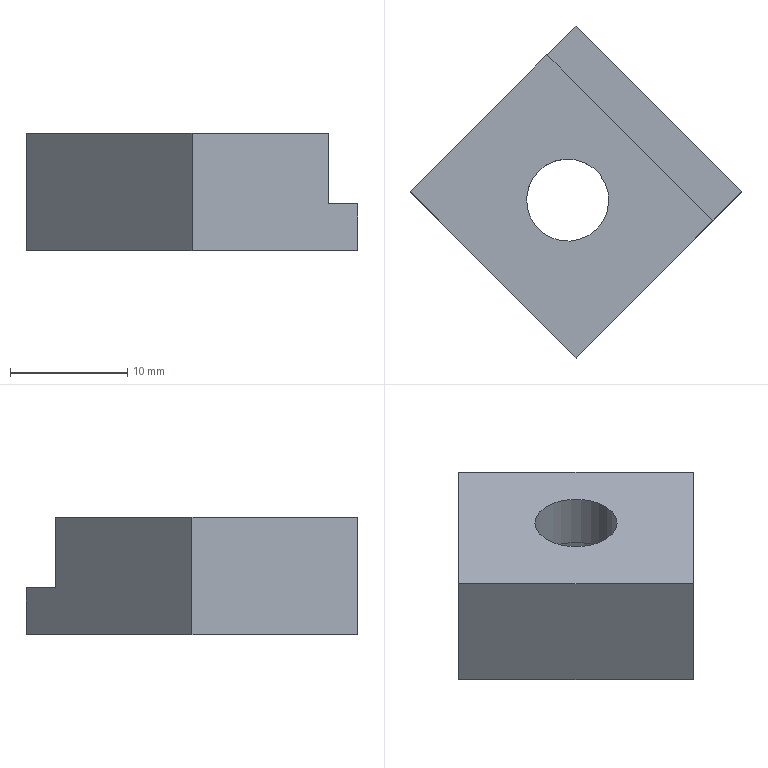Part | 1 solid | 13 faces | box 28.284 x 28.284 x 10 mm | volume 2884 mm3 | plane 9 | cylinder 4 | commonest cylinder face diameters 7 x2 11 x2
STEP:
#1=CARTESIAN_POINT('',(0.,0.,0.));
#2=DIRECTION('',(0.,0.,1.));
#3=DIRECTION('',(1.,0.,0.));
#4=AXIS2_PLACEMENT_3D('',#1,#2,#3);
#5=CARTESIAN_POINT('',(-358.688,26.59,-133.051));
#6=VERTEX_POINT('',#5);
#7=CARTESIAN_POINT('',(-350.91,18.812,-133.051));
#8=VERTEX_POINT('',#7);
#9=CARTESIAN_POINT('',(-354.799,22.701,-133.051));
#10=DIRECTION('',(0.,0.,1.));
#11=DIRECTION('',(-0.7071,0.7071,0.));
#12=AXIS2_PLACEMENT_3D('',#9,#10,#11);
#13=CIRCLE('',#12,5.5);
#14=CARTESIAN_POINT('',(-368.234,23.408,-133.051));
#15=DIRECTION('',(0.,0.,1.));
#16=DIRECTION('',(-0.7071,0.7071,0.));
#17=AXIS2_PLACEMENT_3D('',#14,#15,#16);
#18=PLANE('',#17);
#19=CARTESIAN_POINT('',(-10.,-9.));
#20=DIRECTION('',(1.,0.));
#21=AXIS2_PLACEMENT_2D('',#19,#20);
#22=CIRCLE('',#21,5.5);
#23=(GEOMETRIC_REPRESENTATION_CONTEXT(2)PARAMETRIC_REPRESENTATION_CONTEXT()REPRESENTATION_CONTEXT('',''));
#24=DEFINITIONAL_REPRESENTATION('',(#22),#23);
#25=PCURVE('',#18,#24);
#26=CARTESIAN_POINT('',(-354.799,22.701,-139.051));
#27=DIRECTION('',(0.,0.,1.));
#28=DIRECTION('',(0.7071,0.7071,0.));
#29=AXIS2_PLACEMENT_3D('',#26,#27,#28);
#30=CYLINDRICAL_SURFACE('',#29,5.5);
#31=CARTESIAN_POINT('',(1.571,6.));
#32=DIRECTION('',(1.,0.));
#33=VECTOR('',#32,1.);
#34=LINE('',#31,#33);
#35=(GEOMETRIC_REPRESENTATION_CONTEXT(2)PARAMETRIC_REPRESENTATION_CONTEXT()REPRESENTATION_CONTEXT('',''));
#36=DEFINITIONAL_REPRESENTATION('',(#34),#35);
#37=PCURVE('',#30,#36);
#38=SURFACE_CURVE('',#13,(#25,#37),.PCURVE_S1.);
#39=EDGE_CURVE('',#6,#8,#38,.T.);
#40=ORIENTED_EDGE('',*,*,#39,.T.);
#41=CARTESIAN_POINT('',(-354.799,22.701,-133.051));
#42=DIRECTION('',(0.,0.,1.));
#43=DIRECTION('',(-0.7071,0.7071,0.));
#44=AXIS2_PLACEMENT_3D('',#41,#42,#43);
#45=CIRCLE('',#44,5.5);
#46=CARTESIAN_POINT('',(-10.,-9.));
#47=DIRECTION('',(1.,0.));
#48=AXIS2_PLACEMENT_2D('',#46,#47);
#49=CIRCLE('',#48,5.5);
#50=(GEOMETRIC_REPRESENTATION_CONTEXT(2)PARAMETRIC_REPRESENTATION_CONTEXT()REPRESENTATION_CONTEXT('',''));
#51=DEFINITIONAL_REPRESENTATION('',(#49),#50);
#52=PCURVE('',#18,#51);
#53=CARTESIAN_POINT('',(-354.799,22.701,-139.051));
#54=DIRECTION('',(0.,0.,1.));
#55=DIRECTION('',(-0.7071,-0.7071,0.));
#56=AXIS2_PLACEMENT_3D('',#53,#54,#55);
#57=CYLINDRICAL_SURFACE('',#56,5.5);
#58=CARTESIAN_POINT('',(-1.571,6.));
#59=DIRECTION('',(1.,0.));
#60=VECTOR('',#59,1.);
#61=LINE('',#58,#60);
#62=(GEOMETRIC_REPRESENTATION_CONTEXT(2)PARAMETRIC_REPRESENTATION_CONTEXT()REPRESENTATION_CONTEXT('',''));
#63=DEFINITIONAL_REPRESENTATION('',(#61),#62);
#64=PCURVE('',#57,#63);
#65=SURFACE_CURVE('',#45,(#52,#64),.PCURVE_S1.);
#66=EDGE_CURVE('',#8,#6,#65,.T.);
#67=ORIENTED_EDGE('',*,*,#66,.T.);
#68=EDGE_LOOP('',(#40,#67));
#69=FACE_BOUND('',#68,.T.);
#70=CARTESIAN_POINT('',(-339.95,23.408,-133.051));
#71=VERTEX_POINT('',#70);
#72=CARTESIAN_POINT('',(-354.092,9.266,-133.051));
#73=VERTEX_POINT('',#72);
#74=CARTESIAN_POINT('',(-354.092,9.266,-133.051));
#75=DIRECTION('',(-0.7071,-0.7071,0.));
#76=VECTOR('',#75,1.);
#77=LINE('',#74,#76);
#78=CARTESIAN_POINT('',(-20.,0.));
#79=DIRECTION('',(0.,1.));
#80=VECTOR('',#79,1.);
#81=LINE('',#78,#80);
#82=(GEOMETRIC_REPRESENTATION_CONTEXT(2)PARAMETRIC_REPRESENTATION_CONTEXT()REPRESENTATION_CONTEXT('',''));
#83=DEFINITIONAL_REPRESENTATION('',(#81),#82);
#84=PCURVE('',#18,#83);
#85=CARTESIAN_POINT('',(1570.788,1934.145,521.628));
#86=DIRECTION('',(-0.7071,0.7071,0.));
#87=DIRECTION('',(0.7071,0.7071,0.));
#88=AXIS2_PLACEMENT_3D('',#85,#86,#87);
#89=PLANE('',#88);
#90=CARTESIAN_POINT('',(-2722.191,654.68));
#91=DIRECTION('',(-1.,0.));
#92=VECTOR('',#91,1.);
#93=LINE('',#90,#92);
#94=(GEOMETRIC_REPRESENTATION_CONTEXT(2)PARAMETRIC_REPRESENTATION_CONTEXT()REPRESENTATION_CONTEXT('',''));
#95=DEFINITIONAL_REPRESENTATION('',(#93),#94);
#96=PCURVE('',#89,#95);
#97=SURFACE_CURVE('',#77,(#84,#96),.PCURVE_S1.);
#98=EDGE_CURVE('',#71,#73,#97,.T.);
#99=ORIENTED_EDGE('',*,*,#98,.T.);
#100=CARTESIAN_POINT('',(-368.234,23.408,-133.051));
#101=VERTEX_POINT('',#100);
#102=CARTESIAN_POINT('',(-368.234,23.408,-133.051));
#103=DIRECTION('',(-0.7071,0.7071,0.));
#104=VECTOR('',#103,1.);
#105=LINE('',#102,#104);
#106=CARTESIAN_POINT('',(0.,0.));
#107=DIRECTION('',(1.,0.));
#108=VECTOR('',#107,1.);
#109=LINE('',#106,#108);
#110=(GEOMETRIC_REPRESENTATION_CONTEXT(2)PARAMETRIC_REPRESENTATION_CONTEXT()REPRESENTATION_CONTEXT('',''));
#111=DEFINITIONAL_REPRESENTATION('',(#109),#110);
#112=PCURVE('',#18,#111);
#113=CARTESIAN_POINT('',(-368.234,23.408,-123.051));
#114=DIRECTION('',(0.7071,0.7071,0.));
#115=DIRECTION('',(0.7071,-0.7071,0.));
#116=AXIS2_PLACEMENT_3D('',#113,#114,#115);
#117=PLANE('',#116);
#118=CARTESIAN_POINT('',(0.,10.));
#119=DIRECTION('',(-1.,0.));
#120=VECTOR('',#119,1.);
#121=LINE('',#118,#120);
#122=(GEOMETRIC_REPRESENTATION_CONTEXT(2)PARAMETRIC_REPRESENTATION_CONTEXT()REPRESENTATION_CONTEXT('',''));
#123=DEFINITIONAL_REPRESENTATION('',(#121),#122);
#124=PCURVE('',#117,#123);
#125=SURFACE_CURVE('',#105,(#112,#124),.PCURVE_S1.);
#126=EDGE_CURVE('',#73,#101,#125,.T.);
#127=ORIENTED_EDGE('',*,*,#126,.T.);
#128=CARTESIAN_POINT('',(-354.092,37.55,-133.051));
#129=VERTEX_POINT('',#128);
#130=CARTESIAN_POINT('',(-368.234,23.408,-133.051));
#131=DIRECTION('',(-0.7071,-0.7071,0.));
#132=VECTOR('',#131,1.);
#133=LINE('',#130,#132);
#134=CARTESIAN_POINT('',(0.,0.));
#135=DIRECTION('',(0.,1.));
#136=VECTOR('',#135,1.);
#137=LINE('',#134,#136);
#138=(GEOMETRIC_REPRESENTATION_CONTEXT(2)PARAMETRIC_REPRESENTATION_CONTEXT()REPRESENTATION_CONTEXT('',''));
#139=DEFINITIONAL_REPRESENTATION('',(#137),#138);
#140=PCURVE('',#18,#139);
#141=CARTESIAN_POINT('',(1556.646,1948.287,521.628));
#142=DIRECTION('',(-0.7071,0.7071,0.));
#143=DIRECTION('',(0.7071,0.7071,0.));
#144=AXIS2_PLACEMENT_3D('',#141,#142,#143);
#145=PLANE('',#144);
#146=CARTESIAN_POINT('',(-2722.191,654.68));
#147=DIRECTION('',(-1.,0.));
#148=VECTOR('',#147,1.);
#149=LINE('',#146,#148);
#150=(GEOMETRIC_REPRESENTATION_CONTEXT(2)PARAMETRIC_REPRESENTATION_CONTEXT()REPRESENTATION_CONTEXT('',''));
#151=DEFINITIONAL_REPRESENTATION('',(#149),#150);
#152=PCURVE('',#145,#151);
#153=SURFACE_CURVE('',#133,(#140,#152),.PCURVE_S1.);
#154=EDGE_CURVE('',#129,#101,#153,.T.);
#155=ORIENTED_EDGE('',*,*,#154,.F.);
#156=CARTESIAN_POINT('',(-354.092,37.55,-133.051));
#157=DIRECTION('',(-0.7071,0.7071,0.));
#158=VECTOR('',#157,1.);
#159=LINE('',#156,#158);
#160=CARTESIAN_POINT('',(0.,-20.));
#161=DIRECTION('',(1.,0.));
#162=VECTOR('',#161,1.);
#163=LINE('',#160,#162);
#164=(GEOMETRIC_REPRESENTATION_CONTEXT(2)PARAMETRIC_REPRESENTATION_CONTEXT()REPRESENTATION_CONTEXT('',''));
#165=DEFINITIONAL_REPRESENTATION('',(#163),#164);
#166=PCURVE('',#18,#165);
#167=CARTESIAN_POINT('',(-354.092,37.55,-133.051));
#168=DIRECTION('',(-0.7071,-0.7071,0.));
#169=DIRECTION('',(-0.7071,0.7071,0.));
#170=AXIS2_PLACEMENT_3D('',#167,#168,#169);
#171=PLANE('',#170);
#172=CARTESIAN_POINT('',(0.,0.));
#173=DIRECTION('',(1.,0.));
#174=VECTOR('',#173,1.);
#175=LINE('',#172,#174);
#176=(GEOMETRIC_REPRESENTATION_CONTEXT(2)PARAMETRIC_REPRESENTATION_CONTEXT()REPRESENTATION_CONTEXT('',''));
#177=DEFINITIONAL_REPRESENTATION('',(#175),#176);
#178=PCURVE('',#171,#177);
#179=SURFACE_CURVE('',#159,(#166,#178),.PCURVE_S1.);
#180=EDGE_CURVE('',#71,#129,#179,.T.);
#181=ORIENTED_EDGE('',*,*,#180,.F.);
#182=EDGE_LOOP('',(#99,#127,#155,#181));
#183=FACE_BOUND('',#182,.T.);
#184=ADVANCED_FACE('',(#69,#183),#18,.F.);
#185=CARTESIAN_POINT('',(-339.95,23.408,-129.051));
#186=VERTEX_POINT('',#185);
#187=CARTESIAN_POINT('',(-339.95,23.408,-133.051));
#188=DIRECTION('',(0.,0.,-1.));
#189=VECTOR('',#188,1.);
#190=LINE('',#187,#189);
#191=CARTESIAN_POINT('',(-20.,0.));
#192=DIRECTION('',(0.,1.));
#193=VECTOR('',#192,1.);
#194=LINE('',#191,#193);
#195=(GEOMETRIC_REPRESENTATION_CONTEXT(2)PARAMETRIC_REPRESENTATION_CONTEXT()REPRESENTATION_CONTEXT('',''));
#196=DEFINITIONAL_REPRESENTATION('',(#194),#195);
#197=PCURVE('',#171,#196);
#198=CARTESIAN_POINT('',(-2702.191,654.68));
#199=DIRECTION('',(0.,1.));
#200=VECTOR('',#199,1.);
#201=LINE('',#198,#200);
#202=(GEOMETRIC_REPRESENTATION_CONTEXT(2)PARAMETRIC_REPRESENTATION_CONTEXT()REPRESENTATION_CONTEXT('',''));
#203=DEFINITIONAL_REPRESENTATION('',(#201),#202);
#204=PCURVE('',#89,#203);
#205=SURFACE_CURVE('',#190,(#197,#204),.PCURVE_S1.);
#206=EDGE_CURVE('',#186,#71,#205,.T.);
#207=ORIENTED_EDGE('',*,*,#206,.T.);
#208=ORIENTED_EDGE('',*,*,#180,.T.);
#209=CARTESIAN_POINT('',(-354.092,37.55,-129.051));
#210=VERTEX_POINT('',#209);
#211=CARTESIAN_POINT('',(-354.092,37.55,-133.051));
#212=DIRECTION('',(0.,0.,-1.));
#213=VECTOR('',#212,1.);
#214=LINE('',#211,#213);
#215=CARTESIAN_POINT('',(0.,0.));
#216=DIRECTION('',(0.,1.));
#217=VECTOR('',#216,1.);
#218=LINE('',#215,#217);
#219=(GEOMETRIC_REPRESENTATION_CONTEXT(2)PARAMETRIC_REPRESENTATION_CONTEXT()REPRESENTATION_CONTEXT('',''));
#220=DEFINITIONAL_REPRESENTATION('',(#218),#219);
#221=PCURVE('',#171,#220);
#222=CARTESIAN_POINT('',(-2702.191,654.68));
#223=DIRECTION('',(0.,1.));
#224=VECTOR('',#223,1.);
#225=LINE('',#222,#224);
#226=(GEOMETRIC_REPRESENTATION_CONTEXT(2)PARAMETRIC_REPRESENTATION_CONTEXT()REPRESENTATION_CONTEXT('',''));
#227=DEFINITIONAL_REPRESENTATION('',(#225),#226);
#228=PCURVE('',#145,#227);
#229=SURFACE_CURVE('',#214,(#221,#228),.PCURVE_S1.);
#230=EDGE_CURVE('',#210,#129,#229,.T.);
#231=ORIENTED_EDGE('',*,*,#230,.F.);
#232=CARTESIAN_POINT('',(-354.092,37.55,-129.051));
#233=DIRECTION('',(-0.7071,0.7071,0.));
#234=VECTOR('',#233,1.);
#235=LINE('',#232,#234);
#236=CARTESIAN_POINT('',(0.,-4.));
#237=DIRECTION('',(1.,0.));
#238=VECTOR('',#237,1.);
#239=LINE('',#236,#238);
#240=(GEOMETRIC_REPRESENTATION_CONTEXT(2)PARAMETRIC_REPRESENTATION_CONTEXT()REPRESENTATION_CONTEXT('',''));
#241=DEFINITIONAL_REPRESENTATION('',(#239),#240);
#242=PCURVE('',#171,#241);
#243=CARTESIAN_POINT('',(-354.092,37.55,-129.051));
#244=DIRECTION('',(0.,0.,-1.));
#245=DIRECTION('',(0.7071,-0.7071,0.));
#246=AXIS2_PLACEMENT_3D('',#243,#244,#245);
#247=PLANE('',#246);
#248=CARTESIAN_POINT('',(0.,0.));
#249=DIRECTION('',(-1.,0.));
#250=VECTOR('',#249,1.);
#251=LINE('',#248,#250);
#252=(GEOMETRIC_REPRESENTATION_CONTEXT(2)PARAMETRIC_REPRESENTATION_CONTEXT()REPRESENTATION_CONTEXT('',''));
#253=DEFINITIONAL_REPRESENTATION('',(#251),#252);
#254=PCURVE('',#247,#253);
#255=SURFACE_CURVE('',#235,(#242,#254),.PCURVE_S1.);
#256=EDGE_CURVE('',#186,#210,#255,.T.);
#257=ORIENTED_EDGE('',*,*,#256,.F.);
#258=EDGE_LOOP('',(#207,#208,#231,#257));
#259=FACE_BOUND('',#258,.T.);
#260=ADVANCED_FACE('',(#259),#171,.F.);
#261=CARTESIAN_POINT('',(-342.424,20.933,-129.051));
#262=VERTEX_POINT('',#261);
#263=CARTESIAN_POINT('',(-339.95,23.408,-129.051));
#264=DIRECTION('',(0.7071,0.7071,0.));
#265=VECTOR('',#264,1.);
#266=LINE('',#263,#265);
#267=CARTESIAN_POINT('',(20.,0.));
#268=DIRECTION('',(0.,-1.));
#269=VECTOR('',#268,1.);
#270=LINE('',#267,#269);
#271=(GEOMETRIC_REPRESENTATION_CONTEXT(2)PARAMETRIC_REPRESENTATION_CONTEXT()REPRESENTATION_CONTEXT('',''));
#272=DEFINITIONAL_REPRESENTATION('',(#270),#271);
#273=PCURVE('',#247,#272);
#274=CARTESIAN_POINT('',(-2702.191,650.68));
#275=DIRECTION('',(1.,0.));
#276=VECTOR('',#275,1.);
#277=LINE('',#274,#276);
#278=(GEOMETRIC_REPRESENTATION_CONTEXT(2)PARAMETRIC_REPRESENTATION_CONTEXT()REPRESENTATION_CONTEXT('',''));
#279=DEFINITIONAL_REPRESENTATION('',(#277),#278);
#280=PCURVE('',#89,#279);
#281=SURFACE_CURVE('',#266,(#273,#280),.PCURVE_S1.);
#282=EDGE_CURVE('',#262,#186,#281,.T.);
#283=ORIENTED_EDGE('',*,*,#282,.T.);
#284=ORIENTED_EDGE('',*,*,#256,.T.);
#285=CARTESIAN_POINT('',(-356.567,35.075,-129.051));
#286=VERTEX_POINT('',#285);
#287=CARTESIAN_POINT('',(-354.092,37.55,-129.051));
#288=DIRECTION('',(0.7071,0.7071,0.));
#289=VECTOR('',#288,1.);
#290=LINE('',#287,#289);
#291=CARTESIAN_POINT('',(0.,0.));
#292=DIRECTION('',(0.,-1.));
#293=VECTOR('',#292,1.);
#294=LINE('',#291,#293);
#295=(GEOMETRIC_REPRESENTATION_CONTEXT(2)PARAMETRIC_REPRESENTATION_CONTEXT()REPRESENTATION_CONTEXT('',''));
#296=DEFINITIONAL_REPRESENTATION('',(#294),#295);
#297=PCURVE('',#247,#296);
#298=CARTESIAN_POINT('',(-2702.191,650.68));
#299=DIRECTION('',(1.,0.));
#300=VECTOR('',#299,1.);
#301=LINE('',#298,#300);
#302=(GEOMETRIC_REPRESENTATION_CONTEXT(2)PARAMETRIC_REPRESENTATION_CONTEXT()REPRESENTATION_CONTEXT('',''));
#303=DEFINITIONAL_REPRESENTATION('',(#301),#302);
#304=PCURVE('',#145,#303);
#305=SURFACE_CURVE('',#290,(#297,#304),.PCURVE_S1.);
#306=EDGE_CURVE('',#286,#210,#305,.T.);
#307=ORIENTED_EDGE('',*,*,#306,.F.);
#308=CARTESIAN_POINT('',(-356.567,35.075,-129.051));
#309=DIRECTION('',(-0.7071,0.7071,0.));
#310=VECTOR('',#309,1.);
#311=LINE('',#308,#310);
#312=CARTESIAN_POINT('',(0.,3.5));
#313=DIRECTION('',(-1.,0.));
#314=VECTOR('',#313,1.);
#315=LINE('',#312,#314);
#316=(GEOMETRIC_REPRESENTATION_CONTEXT(2)PARAMETRIC_REPRESENTATION_CONTEXT()REPRESENTATION_CONTEXT('',''));
#317=DEFINITIONAL_REPRESENTATION('',(#315),#316);
#318=PCURVE('',#247,#317);
#319=CARTESIAN_POINT('',(-356.567,35.075,-129.051));
#320=DIRECTION('',(-0.7071,-0.7071,0.));
#321=DIRECTION('',(-0.7071,0.7071,0.));
#322=AXIS2_PLACEMENT_3D('',#319,#320,#321);
#323=PLANE('',#322);
#324=CARTESIAN_POINT('',(0.,0.));
#325=DIRECTION('',(1.,0.));
#326=VECTOR('',#325,1.);
#327=LINE('',#324,#326);
#328=(GEOMETRIC_REPRESENTATION_CONTEXT(2)PARAMETRIC_REPRESENTATION_CONTEXT()REPRESENTATION_CONTEXT('',''));
#329=DEFINITIONAL_REPRESENTATION('',(#327),#328);
#330=PCURVE('',#323,#329);
#331=SURFACE_CURVE('',#311,(#318,#330),.PCURVE_S1.);
#332=EDGE_CURVE('',#262,#286,#331,.T.);
#333=ORIENTED_EDGE('',*,*,#332,.F.);
#334=EDGE_LOOP('',(#283,#284,#307,#333));
#335=FACE_BOUND('',#334,.T.);
#336=ADVANCED_FACE('',(#335),#247,.F.);
#337=CARTESIAN_POINT('',(-342.424,20.933,-123.051));
#338=VERTEX_POINT('',#337);
#339=CARTESIAN_POINT('',(-342.424,20.933,-129.051));
#340=DIRECTION('',(0.,0.,-1.));
#341=VECTOR('',#340,1.);
#342=LINE('',#339,#341);
#343=CARTESIAN_POINT('',(-20.,0.));
#344=DIRECTION('',(0.,1.));
#345=VECTOR('',#344,1.);
#346=LINE('',#343,#345);
#347=(GEOMETRIC_REPRESENTATION_CONTEXT(2)PARAMETRIC_REPRESENTATION_CONTEXT()REPRESENTATION_CONTEXT('',''));
#348=DEFINITIONAL_REPRESENTATION('',(#346),#347);
#349=PCURVE('',#323,#348);
#350=CARTESIAN_POINT('',(-2705.691,650.68));
#351=DIRECTION('',(0.,1.));
#352=VECTOR('',#351,1.);
#353=LINE('',#350,#352);
#354=(GEOMETRIC_REPRESENTATION_CONTEXT(2)PARAMETRIC_REPRESENTATION_CONTEXT()REPRESENTATION_CONTEXT('',''));
#355=DEFINITIONAL_REPRESENTATION('',(#353),#354);
#356=PCURVE('',#89,#355);
#357=SURFACE_CURVE('',#342,(#349,#356),.PCURVE_S1.);
#358=EDGE_CURVE('',#338,#262,#357,.T.);
#359=ORIENTED_EDGE('',*,*,#358,.T.);
#360=ORIENTED_EDGE('',*,*,#332,.T.);
#361=CARTESIAN_POINT('',(-356.567,35.075,-123.051));
#362=VERTEX_POINT('',#361);
#363=CARTESIAN_POINT('',(-356.567,35.075,-129.051));
#364=DIRECTION('',(0.,0.,-1.));
#365=VECTOR('',#364,1.);
#366=LINE('',#363,#365);
#367=CARTESIAN_POINT('',(0.,0.));
#368=DIRECTION('',(0.,1.));
#369=VECTOR('',#368,1.);
#370=LINE('',#367,#369);
#371=(GEOMETRIC_REPRESENTATION_CONTEXT(2)PARAMETRIC_REPRESENTATION_CONTEXT()REPRESENTATION_CONTEXT('',''));
#372=DEFINITIONAL_REPRESENTATION('',(#370),#371);
#373=PCURVE('',#323,#372);
#374=CARTESIAN_POINT('',(-2705.691,650.68));
#375=DIRECTION('',(0.,1.));
#376=VECTOR('',#375,1.);
#377=LINE('',#374,#376);
#378=(GEOMETRIC_REPRESENTATION_CONTEXT(2)PARAMETRIC_REPRESENTATION_CONTEXT()REPRESENTATION_CONTEXT('',''));
#379=DEFINITIONAL_REPRESENTATION('',(#377),#378);
#380=PCURVE('',#145,#379);
#381=SURFACE_CURVE('',#366,(#373,#380),.PCURVE_S1.);
#382=EDGE_CURVE('',#362,#286,#381,.T.);
#383=ORIENTED_EDGE('',*,*,#382,.F.);
#384=CARTESIAN_POINT('',(-356.567,35.075,-123.051));
#385=DIRECTION('',(-0.7071,0.7071,0.));
#386=VECTOR('',#385,1.);
#387=LINE('',#384,#386);
#388=CARTESIAN_POINT('',(0.,-6.));
#389=DIRECTION('',(1.,0.));
#390=VECTOR('',#389,1.);
#391=LINE('',#388,#390);
#392=(GEOMETRIC_REPRESENTATION_CONTEXT(2)PARAMETRIC_REPRESENTATION_CONTEXT()REPRESENTATION_CONTEXT('',''));
#393=DEFINITIONAL_REPRESENTATION('',(#391),#392);
#394=PCURVE('',#323,#393);
#395=CARTESIAN_POINT('',(-356.567,35.075,-123.051));
#396=DIRECTION('',(0.,0.,-1.));
#397=DIRECTION('',(0.7071,-0.7071,0.));
#398=AXIS2_PLACEMENT_3D('',#395,#396,#397);
#399=PLANE('',#398);
#400=CARTESIAN_POINT('',(0.,0.));
#401=DIRECTION('',(-1.,0.));
#402=VECTOR('',#401,1.);
#403=LINE('',#400,#402);
#404=(GEOMETRIC_REPRESENTATION_CONTEXT(2)PARAMETRIC_REPRESENTATION_CONTEXT()REPRESENTATION_CONTEXT('',''));
#405=DEFINITIONAL_REPRESENTATION('',(#403),#404);
#406=PCURVE('',#399,#405);
#407=SURFACE_CURVE('',#387,(#394,#406),.PCURVE_S1.);
#408=EDGE_CURVE('',#338,#362,#407,.T.);
#409=ORIENTED_EDGE('',*,*,#408,.F.);
#410=EDGE_LOOP('',(#359,#360,#383,#409));
#411=FACE_BOUND('',#410,.T.);
#412=ADVANCED_FACE('',(#411),#323,.F.);
#413=CARTESIAN_POINT('',(-357.274,25.176,-123.051));
#414=VERTEX_POINT('',#413);
#415=CARTESIAN_POINT('',(-352.324,20.226,-123.051));
#416=VERTEX_POINT('',#415);
#417=CARTESIAN_POINT('',(-354.799,22.701,-123.051));
#418=DIRECTION('',(0.,0.,-1.));
#419=DIRECTION('',(-0.7071,0.7071,0.));
#420=AXIS2_PLACEMENT_3D('',#417,#418,#419);
#421=CIRCLE('',#420,3.5);
#422=CARTESIAN_POINT('',(10.,7.5));
#423=DIRECTION('',(-1.,0.));
#424=AXIS2_PLACEMENT_2D('',#422,#423);
#425=CIRCLE('',#424,3.5);
#426=(GEOMETRIC_REPRESENTATION_CONTEXT(2)PARAMETRIC_REPRESENTATION_CONTEXT()REPRESENTATION_CONTEXT('',''));
#427=DEFINITIONAL_REPRESENTATION('',(#425),#426);
#428=PCURVE('',#399,#427);
#429=CARTESIAN_POINT('',(-354.799,22.701,-39.051));
#430=DIRECTION('',(0.,0.,1.));
#431=DIRECTION('',(-0.7071,-0.7071,0.));
#432=AXIS2_PLACEMENT_3D('',#429,#430,#431);
#433=CYLINDRICAL_SURFACE('',#432,3.5);
#434=CARTESIAN_POINT('',(4.712,-84.));
#435=DIRECTION('',(-1.,0.));
#436=VECTOR('',#435,1.);
#437=LINE('',#434,#436);
#438=(GEOMETRIC_REPRESENTATION_CONTEXT(2)PARAMETRIC_REPRESENTATION_CONTEXT()REPRESENTATION_CONTEXT('',''));
#439=DEFINITIONAL_REPRESENTATION('',(#437),#438);
#440=PCURVE('',#433,#439);
#441=SURFACE_CURVE('',#421,(#428,#440),.PCURVE_S1.);
#442=EDGE_CURVE('',#414,#416,#441,.T.);
#443=ORIENTED_EDGE('',*,*,#442,.T.);
#444=CARTESIAN_POINT('',(-354.799,22.701,-123.051));
#445=DIRECTION('',(0.,0.,-1.));
#446=DIRECTION('',(-0.7071,0.7071,0.));
#447=AXIS2_PLACEMENT_3D('',#444,#445,#446);
#448=CIRCLE('',#447,3.5);
#449=CARTESIAN_POINT('',(10.,7.5));
#450=DIRECTION('',(-1.,0.));
#451=AXIS2_PLACEMENT_2D('',#449,#450);
#452=CIRCLE('',#451,3.5);
#453=(GEOMETRIC_REPRESENTATION_CONTEXT(2)PARAMETRIC_REPRESENTATION_CONTEXT()REPRESENTATION_CONTEXT('',''));
#454=DEFINITIONAL_REPRESENTATION('',(#452),#453);
#455=PCURVE('',#399,#454);
#456=CARTESIAN_POINT('',(-354.799,22.701,-39.051));
#457=DIRECTION('',(0.,0.,1.));
#458=DIRECTION('',(0.7071,0.7071,0.));
#459=AXIS2_PLACEMENT_3D('',#456,#457,#458);
#460=CYLINDRICAL_SURFACE('',#459,3.5);
#461=CARTESIAN_POINT('',(7.854,-84.));
#462=DIRECTION('',(-1.,0.));
#463=VECTOR('',#462,1.);
#464=LINE('',#461,#463);
#465=(GEOMETRIC_REPRESENTATION_CONTEXT(2)PARAMETRIC_REPRESENTATION_CONTEXT()REPRESENTATION_CONTEXT('',''));
#466=DEFINITIONAL_REPRESENTATION('',(#464),#465);
#467=PCURVE('',#460,#466);
#468=SURFACE_CURVE('',#448,(#455,#467),.PCURVE_S1.);
#469=EDGE_CURVE('',#416,#414,#468,.T.);
#470=ORIENTED_EDGE('',*,*,#469,.T.);
#471=EDGE_LOOP('',(#443,#470));
#472=FACE_BOUND('',#471,.T.);
#473=CARTESIAN_POINT('',(-354.092,9.266,-123.051));
#474=VERTEX_POINT('',#473);
#475=CARTESIAN_POINT('',(-342.424,20.933,-123.051));
#476=DIRECTION('',(0.7071,0.7071,0.));
#477=VECTOR('',#476,1.);
#478=LINE('',#475,#477);
#479=CARTESIAN_POINT('',(20.,0.));
#480=DIRECTION('',(0.,-1.));
#481=VECTOR('',#480,1.);
#482=LINE('',#479,#481);
#483=(GEOMETRIC_REPRESENTATION_CONTEXT(2)PARAMETRIC_REPRESENTATION_CONTEXT()REPRESENTATION_CONTEXT('',''));
#484=DEFINITIONAL_REPRESENTATION('',(#482),#483);
#485=PCURVE('',#399,#484);
#486=CARTESIAN_POINT('',(-2705.691,644.68));
#487=DIRECTION('',(1.,0.));
#488=VECTOR('',#487,1.);
#489=LINE('',#486,#488);
#490=(GEOMETRIC_REPRESENTATION_CONTEXT(2)PARAMETRIC_REPRESENTATION_CONTEXT()REPRESENTATION_CONTEXT('',''));
#491=DEFINITIONAL_REPRESENTATION('',(#489),#490);
#492=PCURVE('',#89,#491);
#493=SURFACE_CURVE('',#478,(#485,#492),.PCURVE_S1.);
#494=EDGE_CURVE('',#474,#338,#493,.T.);
#495=ORIENTED_EDGE('',*,*,#494,.T.);
#496=ORIENTED_EDGE('',*,*,#408,.T.);
#497=CARTESIAN_POINT('',(-368.234,23.408,-123.051));
#498=VERTEX_POINT('',#497);
#499=CARTESIAN_POINT('',(-356.567,35.075,-123.051));
#500=DIRECTION('',(0.7071,0.7071,0.));
#501=VECTOR('',#500,1.);
#502=LINE('',#499,#501);
#503=CARTESIAN_POINT('',(0.,0.));
#504=DIRECTION('',(0.,-1.));
#505=VECTOR('',#504,1.);
#506=LINE('',#503,#505);
#507=(GEOMETRIC_REPRESENTATION_CONTEXT(2)PARAMETRIC_REPRESENTATION_CONTEXT()REPRESENTATION_CONTEXT('',''));
#508=DEFINITIONAL_REPRESENTATION('',(#506),#507);
#509=PCURVE('',#399,#508);
#510=CARTESIAN_POINT('',(-2705.691,644.68));
#511=DIRECTION('',(1.,0.));
#512=VECTOR('',#511,1.);
#513=LINE('',#510,#512);
#514=(GEOMETRIC_REPRESENTATION_CONTEXT(2)PARAMETRIC_REPRESENTATION_CONTEXT()REPRESENTATION_CONTEXT('',''));
#515=DEFINITIONAL_REPRESENTATION('',(#513),#514);
#516=PCURVE('',#145,#515);
#517=SURFACE_CURVE('',#502,(#509,#516),.PCURVE_S1.);
#518=EDGE_CURVE('',#498,#362,#517,.T.);
#519=ORIENTED_EDGE('',*,*,#518,.F.);
#520=CARTESIAN_POINT('',(-368.234,23.408,-123.051));
#521=DIRECTION('',(-0.7071,0.7071,0.));
#522=VECTOR('',#521,1.);
#523=LINE('',#520,#522);
#524=CARTESIAN_POINT('',(0.,16.5));
#525=DIRECTION('',(-1.,0.));
#526=VECTOR('',#525,1.);
#527=LINE('',#524,#526);
#528=(GEOMETRIC_REPRESENTATION_CONTEXT(2)PARAMETRIC_REPRESENTATION_CONTEXT()REPRESENTATION_CONTEXT('',''));
#529=DEFINITIONAL_REPRESENTATION('',(#527),#528);
#530=PCURVE('',#399,#529);
#531=CARTESIAN_POINT('',(0.,0.));
#532=DIRECTION('',(-1.,0.));
#533=VECTOR('',#532,1.);
#534=LINE('',#531,#533);
#535=(GEOMETRIC_REPRESENTATION_CONTEXT(2)PARAMETRIC_REPRESENTATION_CONTEXT()REPRESENTATION_CONTEXT('',''));
#536=DEFINITIONAL_REPRESENTATION('',(#534),#535);
#537=PCURVE('',#117,#536);
#538=SURFACE_CURVE('',#523,(#530,#537),.PCURVE_S1.);
#539=EDGE_CURVE('',#474,#498,#538,.T.);
#540=ORIENTED_EDGE('',*,*,#539,.F.);
#541=EDGE_LOOP('',(#495,#496,#519,#540));
#542=FACE_BOUND('',#541,.T.);
#543=ADVANCED_FACE('',(#472,#542),#399,.F.);
#544=CARTESIAN_POINT('',(-354.092,9.266,-123.051));
#545=DIRECTION('',(0.,0.,1.));
#546=VECTOR('',#545,1.);
#547=LINE('',#544,#546);
#548=CARTESIAN_POINT('',(20.,0.));
#549=DIRECTION('',(0.,-1.));
#550=VECTOR('',#549,1.);
#551=LINE('',#548,#550);
#552=(GEOMETRIC_REPRESENTATION_CONTEXT(2)PARAMETRIC_REPRESENTATION_CONTEXT()REPRESENTATION_CONTEXT('',''));
#553=DEFINITIONAL_REPRESENTATION('',(#551),#552);
#554=PCURVE('',#117,#553);
#555=CARTESIAN_POINT('',(-2722.191,644.68));
#556=DIRECTION('',(0.,-1.));
#557=VECTOR('',#556,1.);
#558=LINE('',#555,#557);
#559=(GEOMETRIC_REPRESENTATION_CONTEXT(2)PARAMETRIC_REPRESENTATION_CONTEXT()REPRESENTATION_CONTEXT('',''));
#560=DEFINITIONAL_REPRESENTATION('',(#558),#559);
#561=PCURVE('',#89,#560);
#562=SURFACE_CURVE('',#547,(#554,#561),.PCURVE_S1.);
#563=EDGE_CURVE('',#73,#474,#562,.T.);
#564=ORIENTED_EDGE('',*,*,#563,.T.);
#565=ORIENTED_EDGE('',*,*,#539,.T.);
#566=CARTESIAN_POINT('',(-368.234,23.408,-123.051));
#567=DIRECTION('',(0.,0.,1.));
#568=VECTOR('',#567,1.);
#569=LINE('',#566,#568);
#570=CARTESIAN_POINT('',(0.,0.));
#571=DIRECTION('',(0.,-1.));
#572=VECTOR('',#571,1.);
#573=LINE('',#570,#572);
#574=(GEOMETRIC_REPRESENTATION_CONTEXT(2)PARAMETRIC_REPRESENTATION_CONTEXT()REPRESENTATION_CONTEXT('',''));
#575=DEFINITIONAL_REPRESENTATION('',(#573),#574);
#576=PCURVE('',#117,#575);
#577=CARTESIAN_POINT('',(-2722.191,644.68));
#578=DIRECTION('',(0.,-1.));
#579=VECTOR('',#578,1.);
#580=LINE('',#577,#579);
#581=(GEOMETRIC_REPRESENTATION_CONTEXT(2)PARAMETRIC_REPRESENTATION_CONTEXT()REPRESENTATION_CONTEXT('',''));
#582=DEFINITIONAL_REPRESENTATION('',(#580),#581);
#583=PCURVE('',#145,#582);
#584=SURFACE_CURVE('',#569,(#576,#583),.PCURVE_S1.);
#585=EDGE_CURVE('',#101,#498,#584,.T.);
#586=ORIENTED_EDGE('',*,*,#585,.F.);
#587=ORIENTED_EDGE('',*,*,#126,.F.);
#588=EDGE_LOOP('',(#564,#565,#586,#587));
#589=FACE_BOUND('',#588,.T.);
#590=ADVANCED_FACE('',(#589),#117,.F.);
#591=ORIENTED_EDGE('',*,*,#154,.T.);
#592=ORIENTED_EDGE('',*,*,#585,.T.);
#593=ORIENTED_EDGE('',*,*,#518,.T.);
#594=ORIENTED_EDGE('',*,*,#382,.T.);
#595=ORIENTED_EDGE('',*,*,#306,.T.);
#596=ORIENTED_EDGE('',*,*,#230,.T.);
#597=EDGE_LOOP('',(#591,#592,#593,#594,#595,#596));
#598=FACE_BOUND('',#597,.T.);
#599=ADVANCED_FACE('',(#598),#145,.T.);
#600=ORIENTED_EDGE('',*,*,#98,.F.);
#601=ORIENTED_EDGE('',*,*,#206,.F.);
#602=ORIENTED_EDGE('',*,*,#282,.F.);
#603=ORIENTED_EDGE('',*,*,#358,.F.);
#604=ORIENTED_EDGE('',*,*,#494,.F.);
#605=ORIENTED_EDGE('',*,*,#563,.F.);
#606=EDGE_LOOP('',(#600,#601,#602,#603,#604,#605));
#607=FACE_BOUND('',#606,.T.);
#608=ADVANCED_FACE('',(#607),#89,.F.);
#609=CARTESIAN_POINT('',(-357.274,25.176,-127.551));
#610=VERTEX_POINT('',#609);
#611=CARTESIAN_POINT('',(-352.324,20.226,-127.551));
#612=VERTEX_POINT('',#611);
#613=CARTESIAN_POINT('',(-354.799,22.701,-127.551));
#614=DIRECTION('',(0.,0.,-1.));
#615=DIRECTION('',(-0.7071,0.7071,0.));
#616=AXIS2_PLACEMENT_3D('',#613,#614,#615);
#617=CIRCLE('',#616,3.5);
#618=CARTESIAN_POINT('',(4.712,-88.5));
#619=DIRECTION('',(-1.,0.));
#620=VECTOR('',#619,1.);
#621=LINE('',#618,#620);
#622=(GEOMETRIC_REPRESENTATION_CONTEXT(2)PARAMETRIC_REPRESENTATION_CONTEXT()REPRESENTATION_CONTEXT('',''));
#623=DEFINITIONAL_REPRESENTATION('',(#621),#622);
#624=PCURVE('',#433,#623);
#625=CARTESIAN_POINT('',(-354.799,22.701,-127.551));
#626=DIRECTION('',(0.,0.,1.));
#627=DIRECTION('',(-0.7071,0.7071,0.));
#628=AXIS2_PLACEMENT_3D('',#625,#626,#627);
#629=PLANE('',#628);
#630=CARTESIAN_POINT('',(3.5,0.));
#631=CARTESIAN_POINT('',(3.5,-6.062));
#632=CARTESIAN_POINT('',(-1.75,-3.031));
#633=CARTESIAN_POINT('',(-7.,0.));
#634=CARTESIAN_POINT('',(-1.75,3.031));
#635=CARTESIAN_POINT('',(3.5,6.062));
#636=CARTESIAN_POINT('',(3.5,0.));
#637=(BOUNDED_CURVE()B_SPLINE_CURVE(2,(#630,#631,#632,#633,#634,#635,#636),.UNSPECIFIED.,.T.,.F.)B_SPLINE_CURVE_WITH_KNOTS((1,2,2,2,2,1),(-2.094,0.,2.094,4.189,6.283,8.378),.UNSPECIFIED.)CURVE()GEOMETRIC_REPRESENTATION_ITEM()RATIONAL_B_SPLINE_CURVE((1.,0.5,1.,0.5,1.,0.5,1.))REPRESENTATION_ITEM(''));
#638=(GEOMETRIC_REPRESENTATION_CONTEXT(2)PARAMETRIC_REPRESENTATION_CONTEXT()REPRESENTATION_CONTEXT('',''));
#639=DEFINITIONAL_REPRESENTATION('',(#637),#638);
#640=PCURVE('',#629,#639);
#641=SURFACE_CURVE('',#617,(#624,#640),.PCURVE_S1.);
#642=EDGE_CURVE('',#610,#612,#641,.T.);
#643=ORIENTED_EDGE('',*,*,#642,.F.);
#644=CARTESIAN_POINT('',(-357.274,25.176,-127.551));
#645=DIRECTION('',(0.,0.,1.));
#646=VECTOR('',#645,1.);
#647=LINE('',#644,#646);
#648=CARTESIAN_POINT('',(4.712,-88.5));
#649=DIRECTION('',(0.,1.));
#650=VECTOR('',#649,1.);
#651=LINE('',#648,#650);
#652=(GEOMETRIC_REPRESENTATION_CONTEXT(2)PARAMETRIC_REPRESENTATION_CONTEXT()REPRESENTATION_CONTEXT('',''));
#653=DEFINITIONAL_REPRESENTATION('',(#651),#652);
#654=PCURVE('',#433,#653);
#655=CARTESIAN_POINT('',(1.571,-88.5));
#656=DIRECTION('',(0.,1.));
#657=VECTOR('',#656,1.);
#658=LINE('',#655,#657);
#659=(GEOMETRIC_REPRESENTATION_CONTEXT(2)PARAMETRIC_REPRESENTATION_CONTEXT()REPRESENTATION_CONTEXT('',''));
#660=DEFINITIONAL_REPRESENTATION('',(#658),#659);
#661=PCURVE('',#460,#660);
#662=SURFACE_CURVE('',#647,(#654,#661),.PCURVE_S1.);
#663=EDGE_CURVE('',#610,#414,#662,.T.);
#664=ORIENTED_EDGE('',*,*,#663,.T.);
#665=ORIENTED_EDGE('',*,*,#442,.T.);
#666=CARTESIAN_POINT('',(-352.324,20.226,-127.551));
#667=DIRECTION('',(0.,0.,1.));
#668=VECTOR('',#667,1.);
#669=LINE('',#666,#668);
#670=CARTESIAN_POINT('',(1.571,-88.5));
#671=DIRECTION('',(0.,1.));
#672=VECTOR('',#671,1.);
#673=LINE('',#670,#672);
#674=(GEOMETRIC_REPRESENTATION_CONTEXT(2)PARAMETRIC_REPRESENTATION_CONTEXT()REPRESENTATION_CONTEXT('',''));
#675=DEFINITIONAL_REPRESENTATION('',(#673),#674);
#676=PCURVE('',#433,#675);
#677=CARTESIAN_POINT('',(4.712,-88.5));
#678=DIRECTION('',(0.,1.));
#679=VECTOR('',#678,1.);
#680=LINE('',#677,#679);
#681=(GEOMETRIC_REPRESENTATION_CONTEXT(2)PARAMETRIC_REPRESENTATION_CONTEXT()REPRESENTATION_CONTEXT('',''));
#682=DEFINITIONAL_REPRESENTATION('',(#680),#681);
#683=PCURVE('',#460,#682);
#684=SURFACE_CURVE('',#669,(#676,#683),.PCURVE_S1.);
#685=EDGE_CURVE('',#612,#416,#684,.T.);
#686=ORIENTED_EDGE('',*,*,#685,.F.);
#687=EDGE_LOOP('',(#643,#664,#665,#686));
#688=FACE_BOUND('',#687,.F.);
#689=ADVANCED_FACE('',(#688),#433,.F.);
#690=CARTESIAN_POINT('',(-354.799,22.701,-127.551));
#691=DIRECTION('',(0.,0.,-1.));
#692=DIRECTION('',(-0.7071,0.7071,0.));
#693=AXIS2_PLACEMENT_3D('',#690,#691,#692);
#694=CIRCLE('',#693,3.5);
#695=CARTESIAN_POINT('',(3.5,0.));
#696=CARTESIAN_POINT('',(3.5,-6.062));
#697=CARTESIAN_POINT('',(-1.75,-3.031));
#698=CARTESIAN_POINT('',(-7.,0.));
#699=CARTESIAN_POINT('',(-1.75,3.031));
#700=CARTESIAN_POINT('',(3.5,6.062));
#701=CARTESIAN_POINT('',(3.5,0.));
#702=(BOUNDED_CURVE()B_SPLINE_CURVE(2,(#695,#696,#697,#698,#699,#700,#701),.UNSPECIFIED.,.T.,.F.)B_SPLINE_CURVE_WITH_KNOTS((1,2,2,2,2,1),(-2.094,0.,2.094,4.189,6.283,8.378),.UNSPECIFIED.)CURVE()GEOMETRIC_REPRESENTATION_ITEM()RATIONAL_B_SPLINE_CURVE((1.,0.5,1.,0.5,1.,0.5,1.))REPRESENTATION_ITEM(''));
#703=(GEOMETRIC_REPRESENTATION_CONTEXT(2)PARAMETRIC_REPRESENTATION_CONTEXT()REPRESENTATION_CONTEXT('',''));
#704=DEFINITIONAL_REPRESENTATION('',(#702),#703);
#705=PCURVE('',#629,#704);
#706=CARTESIAN_POINT('',(7.854,-88.5));
#707=DIRECTION('',(-1.,0.));
#708=VECTOR('',#707,1.);
#709=LINE('',#706,#708);
#710=(GEOMETRIC_REPRESENTATION_CONTEXT(2)PARAMETRIC_REPRESENTATION_CONTEXT()REPRESENTATION_CONTEXT('',''));
#711=DEFINITIONAL_REPRESENTATION('',(#709),#710);
#712=PCURVE('',#460,#711);
#713=SURFACE_CURVE('',#694,(#705,#712),.PCURVE_S1.);
#714=EDGE_CURVE('',#612,#610,#713,.T.);
#715=ORIENTED_EDGE('',*,*,#714,.F.);
#716=ORIENTED_EDGE('',*,*,#642,.F.);
#717=EDGE_LOOP('',(#715,#716));
#718=FACE_BOUND('',#717,.T.);
#719=CARTESIAN_POINT('',(-358.688,26.59,-127.551));
#720=VERTEX_POINT('',#719);
#721=CARTESIAN_POINT('',(-350.91,18.812,-127.551));
#722=VERTEX_POINT('',#721);
#723=CARTESIAN_POINT('',(-354.799,22.701,-127.551));
#724=DIRECTION('',(0.,0.,-1.));
#725=DIRECTION('',(-0.7071,0.7071,0.));
#726=AXIS2_PLACEMENT_3D('',#723,#724,#725);
#727=CIRCLE('',#726,5.5);
#728=CARTESIAN_POINT('',(5.5,0.));
#729=CARTESIAN_POINT('',(5.5,-9.526));
#730=CARTESIAN_POINT('',(-2.75,-4.763));
#731=CARTESIAN_POINT('',(-11.,0.));
#732=CARTESIAN_POINT('',(-2.75,4.763));
#733=CARTESIAN_POINT('',(5.5,9.526));
#734=CARTESIAN_POINT('',(5.5,0.));
#735=(BOUNDED_CURVE()B_SPLINE_CURVE(2,(#728,#729,#730,#731,#732,#733,#734),.UNSPECIFIED.,.T.,.F.)B_SPLINE_CURVE_WITH_KNOTS((1,2,2,2,2,1),(-2.094,0.,2.094,4.189,6.283,8.378),.UNSPECIFIED.)CURVE()GEOMETRIC_REPRESENTATION_ITEM()RATIONAL_B_SPLINE_CURVE((1.,0.5,1.,0.5,1.,0.5,1.))REPRESENTATION_ITEM(''));
#736=(GEOMETRIC_REPRESENTATION_CONTEXT(2)PARAMETRIC_REPRESENTATION_CONTEXT()REPRESENTATION_CONTEXT('',''));
#737=DEFINITIONAL_REPRESENTATION('',(#735),#736);
#738=PCURVE('',#629,#737);
#739=CARTESIAN_POINT('',(4.712,11.5));
#740=DIRECTION('',(-1.,0.));
#741=VECTOR('',#740,1.);
#742=LINE('',#739,#741);
#743=(GEOMETRIC_REPRESENTATION_CONTEXT(2)PARAMETRIC_REPRESENTATION_CONTEXT()REPRESENTATION_CONTEXT('',''));
#744=DEFINITIONAL_REPRESENTATION('',(#742),#743);
#745=PCURVE('',#57,#744);
#746=SURFACE_CURVE('',#727,(#738,#745),.PCURVE_S1.);
#747=EDGE_CURVE('',#720,#722,#746,.T.);
#748=ORIENTED_EDGE('',*,*,#747,.T.);
#749=CARTESIAN_POINT('',(-354.799,22.701,-127.551));
#750=DIRECTION('',(0.,0.,-1.));
#751=DIRECTION('',(-0.7071,0.7071,0.));
#752=AXIS2_PLACEMENT_3D('',#749,#750,#751);
#753=CIRCLE('',#752,5.5);
#754=CARTESIAN_POINT('',(5.5,0.));
#755=CARTESIAN_POINT('',(5.5,-9.526));
#756=CARTESIAN_POINT('',(-2.75,-4.763));
#757=CARTESIAN_POINT('',(-11.,0.));
#758=CARTESIAN_POINT('',(-2.75,4.763));
#759=CARTESIAN_POINT('',(5.5,9.526));
#760=CARTESIAN_POINT('',(5.5,0.));
#761=(BOUNDED_CURVE()B_SPLINE_CURVE(2,(#754,#755,#756,#757,#758,#759,#760),.UNSPECIFIED.,.T.,.F.)B_SPLINE_CURVE_WITH_KNOTS((1,2,2,2,2,1),(-2.094,0.,2.094,4.189,6.283,8.378),.UNSPECIFIED.)CURVE()GEOMETRIC_REPRESENTATION_ITEM()RATIONAL_B_SPLINE_CURVE((1.,0.5,1.,0.5,1.,0.5,1.))REPRESENTATION_ITEM(''));
#762=(GEOMETRIC_REPRESENTATION_CONTEXT(2)PARAMETRIC_REPRESENTATION_CONTEXT()REPRESENTATION_CONTEXT('',''));
#763=DEFINITIONAL_REPRESENTATION('',(#761),#762);
#764=PCURVE('',#629,#763);
#765=CARTESIAN_POINT('',(7.854,11.5));
#766=DIRECTION('',(-1.,0.));
#767=VECTOR('',#766,1.);
#768=LINE('',#765,#767);
#769=(GEOMETRIC_REPRESENTATION_CONTEXT(2)PARAMETRIC_REPRESENTATION_CONTEXT()REPRESENTATION_CONTEXT('',''));
#770=DEFINITIONAL_REPRESENTATION('',(#768),#769);
#771=PCURVE('',#30,#770);
#772=SURFACE_CURVE('',#753,(#764,#771),.PCURVE_S1.);
#773=EDGE_CURVE('',#722,#720,#772,.T.);
#774=ORIENTED_EDGE('',*,*,#773,.T.);
#775=EDGE_LOOP('',(#748,#774));
#776=FACE_BOUND('',#775,.T.);
#777=ADVANCED_FACE('',(#718,#776),#629,.F.);
#778=ORIENTED_EDGE('',*,*,#66,.T.);
#779=CARTESIAN_POINT('',(-358.688,26.59,-133.051));
#780=DIRECTION('',(0.,0.,1.));
#781=VECTOR('',#780,1.);
#782=LINE('',#779,#781);
#783=CARTESIAN_POINT('',(4.712,6.));
#784=DIRECTION('',(0.,1.));
#785=VECTOR('',#784,1.);
#786=LINE('',#783,#785);
#787=(GEOMETRIC_REPRESENTATION_CONTEXT(2)PARAMETRIC_REPRESENTATION_CONTEXT()REPRESENTATION_CONTEXT('',''));
#788=DEFINITIONAL_REPRESENTATION('',(#786),#787);
#789=PCURVE('',#57,#788);
#790=CARTESIAN_POINT('',(1.571,6.));
#791=DIRECTION('',(0.,1.));
#792=VECTOR('',#791,1.);
#793=LINE('',#790,#792);
#794=(GEOMETRIC_REPRESENTATION_CONTEXT(2)PARAMETRIC_REPRESENTATION_CONTEXT()REPRESENTATION_CONTEXT('',''));
#795=DEFINITIONAL_REPRESENTATION('',(#793),#794);
#796=PCURVE('',#30,#795);
#797=SURFACE_CURVE('',#782,(#789,#796),.PCURVE_S1.);
#798=EDGE_CURVE('',#6,#720,#797,.T.);
#799=ORIENTED_EDGE('',*,*,#798,.T.);
#800=ORIENTED_EDGE('',*,*,#747,.T.);
#801=CARTESIAN_POINT('',(-350.91,18.812,-133.051));
#802=DIRECTION('',(0.,0.,1.));
#803=VECTOR('',#802,1.);
#804=LINE('',#801,#803);
#805=CARTESIAN_POINT('',(1.571,6.));
#806=DIRECTION('',(0.,1.));
#807=VECTOR('',#806,1.);
#808=LINE('',#805,#807);
#809=(GEOMETRIC_REPRESENTATION_CONTEXT(2)PARAMETRIC_REPRESENTATION_CONTEXT()REPRESENTATION_CONTEXT('',''));
#810=DEFINITIONAL_REPRESENTATION('',(#808),#809);
#811=PCURVE('',#57,#810);
#812=CARTESIAN_POINT('',(4.712,6.));
#813=DIRECTION('',(0.,1.));
#814=VECTOR('',#813,1.);
#815=LINE('',#812,#814);
#816=(GEOMETRIC_REPRESENTATION_CONTEXT(2)PARAMETRIC_REPRESENTATION_CONTEXT()REPRESENTATION_CONTEXT('',''));
#817=DEFINITIONAL_REPRESENTATION('',(#815),#816);
#818=PCURVE('',#30,#817);
#819=SURFACE_CURVE('',#804,(#811,#818),.PCURVE_S1.);
#820=EDGE_CURVE('',#8,#722,#819,.T.);
#821=ORIENTED_EDGE('',*,*,#820,.F.);
#822=EDGE_LOOP('',(#778,#799,#800,#821));
#823=FACE_BOUND('',#822,.F.);
#824=ADVANCED_FACE('',(#823),#57,.F.);
#825=ORIENTED_EDGE('',*,*,#469,.T.);
#826=ORIENTED_EDGE('',*,*,#663,.F.);
#827=ORIENTED_EDGE('',*,*,#714,.F.);
#828=ORIENTED_EDGE('',*,*,#685,.T.);
#829=EDGE_LOOP('',(#825,#826,#827,#828));
#830=FACE_BOUND('',#829,.F.);
#831=ADVANCED_FACE('',(#830),#460,.F.);
#832=ORIENTED_EDGE('',*,*,#773,.T.);
#833=ORIENTED_EDGE('',*,*,#798,.F.);
#834=ORIENTED_EDGE('',*,*,#39,.T.);
#835=ORIENTED_EDGE('',*,*,#820,.T.);
#836=EDGE_LOOP('',(#832,#833,#834,#835));
#837=FACE_BOUND('',#836,.F.);
#838=ADVANCED_FACE('',(#837),#30,.F.);
#839=CLOSED_SHELL('',(#184,#260,#336,#412,#543,#590,#599,#608,#689,#777,#824,#831,#838));
#840=MANIFOLD_SOLID_BREP('',#839);
#841=(LENGTH_UNIT()NAMED_UNIT(*)SI_UNIT(.MILLI.,.METRE.));
#842=UNCERTAINTY_MEASURE_WITH_UNIT(LENGTH_MEASURE(0.0000001),#841,'','');
#843=(NAMED_UNIT(*)PLANE_ANGLE_UNIT()SI_UNIT($,.RADIAN.));
#844=(NAMED_UNIT(*)SI_UNIT($,.STERADIAN.)SOLID_ANGLE_UNIT());
#845=(GEOMETRIC_REPRESENTATION_CONTEXT(3)GLOBAL_UNCERTAINTY_ASSIGNED_CONTEXT((#842))GLOBAL_UNIT_ASSIGNED_CONTEXT((#841,#843,#844))REPRESENTATION_CONTEXT('',''));
#846=ADVANCED_BREP_SHAPE_REPRESENTATION('',(#4,#840),#845);